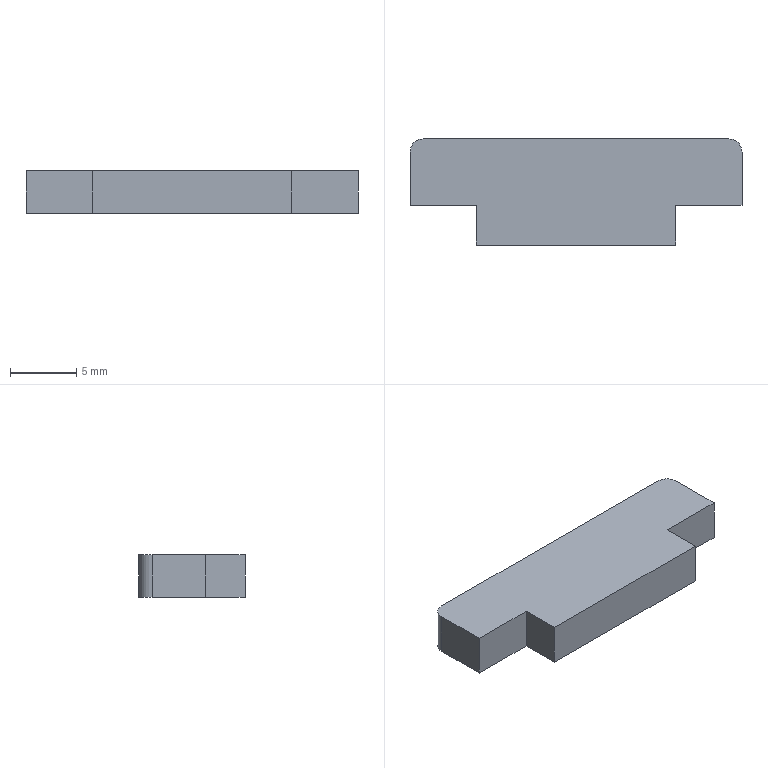Part | SolidWorks | features FlatPattern 1, SMBaseFlange 1, SheetMetal 1 | 1 solid | 12 faces | box 25 x 8 x 3.2 mm | volume 542.627 mm3 | plane 10 | cylinder 2 | commonest cylinder face diameters 2 x2
STEP:
#1=CARTESIAN_POINT('',(100.,-30.,0.));
#2=VERTEX_POINT('',#1);
#3=CARTESIAN_POINT('',(100.,-34.,0.));
#4=VERTEX_POINT('',#3);
#5=CARTESIAN_POINT('',(100.,-34.,0.));
#6=DIRECTION('',(0.,-1.,0.));
#7=VECTOR('',#6,1000.);
#8=LINE('',#5,#7);
#9=EDGE_CURVE('',#2,#4,#8,.T.);
#10=ORIENTED_EDGE('',*,*,#9,.T.);
#11=CARTESIAN_POINT('',(100.,-34.,3.2));
#12=VERTEX_POINT('',#11);
#13=CARTESIAN_POINT('',(100.,-34.,3.2));
#14=DIRECTION('',(0.,0.,-1.));
#15=VECTOR('',#14,1000.);
#16=LINE('',#13,#15);
#17=EDGE_CURVE('',#12,#4,#16,.T.);
#18=ORIENTED_EDGE('',*,*,#17,.F.);
#19=CARTESIAN_POINT('',(100.,-30.,3.2));
#20=VERTEX_POINT('',#19);
#21=CARTESIAN_POINT('',(100.,-34.,3.2));
#22=DIRECTION('',(0.,-1.,0.));
#23=VECTOR('',#22,1000.);
#24=LINE('',#21,#23);
#25=EDGE_CURVE('',#20,#12,#24,.T.);
#26=ORIENTED_EDGE('',*,*,#25,.F.);
#27=CARTESIAN_POINT('',(100.,-30.,3.2));
#28=DIRECTION('',(0.,0.,-1.));
#29=VECTOR('',#28,1000.);
#30=LINE('',#27,#29);
#31=EDGE_CURVE('',#20,#2,#30,.T.);
#32=ORIENTED_EDGE('',*,*,#31,.T.);
#33=EDGE_LOOP('',(#10,#18,#26,#32));
#34=FACE_OUTER_BOUND('',#33,.T.);
#35=CARTESIAN_POINT('',(100.,-34.,3.2));
#36=DIRECTION('',(1.,0.,0.));
#37=DIRECTION('',(0.,0.,-1.));
#38=AXIS2_PLACEMENT_3D('',#35,#36,#37);
#39=PLANE('',#38);
#40=ADVANCED_FACE('',(#34),#39,.F.);
#41=CARTESIAN_POINT('',(105.,-34.,0.));
#42=VERTEX_POINT('',#41);
#43=CARTESIAN_POINT('',(100.,-34.,0.));
#44=DIRECTION('',(1.,0.,0.));
#45=VECTOR('',#44,1000.);
#46=LINE('',#43,#45);
#47=EDGE_CURVE('',#4,#42,#46,.T.);
#48=ORIENTED_EDGE('',*,*,#47,.T.);
#49=CARTESIAN_POINT('',(105.,-34.,3.2));
#50=VERTEX_POINT('',#49);
#51=CARTESIAN_POINT('',(105.,-34.,3.2));
#52=DIRECTION('',(0.,0.,-1.));
#53=VECTOR('',#52,1000.);
#54=LINE('',#51,#53);
#55=EDGE_CURVE('',#50,#42,#54,.T.);
#56=ORIENTED_EDGE('',*,*,#55,.F.);
#57=CARTESIAN_POINT('',(100.,-34.,3.2));
#58=DIRECTION('',(1.,0.,0.));
#59=VECTOR('',#58,1000.);
#60=LINE('',#57,#59);
#61=EDGE_CURVE('',#12,#50,#60,.T.);
#62=ORIENTED_EDGE('',*,*,#61,.F.);
#63=ORIENTED_EDGE('',*,*,#17,.T.);
#64=EDGE_LOOP('',(#48,#56,#62,#63));
#65=FACE_OUTER_BOUND('',#64,.T.);
#66=CARTESIAN_POINT('',(100.,-34.,3.2));
#67=DIRECTION('',(0.,1.,0.));
#68=DIRECTION('',(0.,0.,1.));
#69=AXIS2_PLACEMENT_3D('',#66,#67,#68);
#70=PLANE('',#69);
#71=ADVANCED_FACE('',(#65),#70,.F.);
#72=CARTESIAN_POINT('',(105.,-37.,0.));
#73=VERTEX_POINT('',#72);
#74=CARTESIAN_POINT('',(105.,-34.,0.));
#75=DIRECTION('',(0.,-1.,0.));
#76=VECTOR('',#75,1000.);
#77=LINE('',#74,#76);
#78=EDGE_CURVE('',#42,#73,#77,.T.);
#79=ORIENTED_EDGE('',*,*,#78,.T.);
#80=CARTESIAN_POINT('',(105.,-37.,3.2));
#81=VERTEX_POINT('',#80);
#82=CARTESIAN_POINT('',(105.,-37.,3.2));
#83=DIRECTION('',(0.,0.,-1.));
#84=VECTOR('',#83,1000.);
#85=LINE('',#82,#84);
#86=EDGE_CURVE('',#81,#73,#85,.T.);
#87=ORIENTED_EDGE('',*,*,#86,.F.);
#88=CARTESIAN_POINT('',(105.,-34.,3.2));
#89=DIRECTION('',(0.,-1.,0.));
#90=VECTOR('',#89,1000.);
#91=LINE('',#88,#90);
#92=EDGE_CURVE('',#50,#81,#91,.T.);
#93=ORIENTED_EDGE('',*,*,#92,.F.);
#94=ORIENTED_EDGE('',*,*,#55,.T.);
#95=EDGE_LOOP('',(#79,#87,#93,#94));
#96=FACE_OUTER_BOUND('',#95,.T.);
#97=CARTESIAN_POINT('',(105.,-34.,3.2));
#98=DIRECTION('',(1.,0.,0.));
#99=DIRECTION('',(0.,0.,-1.));
#100=AXIS2_PLACEMENT_3D('',#97,#98,#99);
#101=PLANE('',#100);
#102=ADVANCED_FACE('',(#96),#101,.F.);
#103=CARTESIAN_POINT('',(120.,-37.,0.));
#104=VERTEX_POINT('',#103);
#105=CARTESIAN_POINT('',(105.,-37.,0.));
#106=DIRECTION('',(1.,0.,0.));
#107=VECTOR('',#106,1000.);
#108=LINE('',#105,#107);
#109=EDGE_CURVE('',#73,#104,#108,.T.);
#110=ORIENTED_EDGE('',*,*,#109,.T.);
#111=CARTESIAN_POINT('',(120.,-37.,3.2));
#112=VERTEX_POINT('',#111);
#113=CARTESIAN_POINT('',(120.,-37.,3.2));
#114=DIRECTION('',(0.,0.,-1.));
#115=VECTOR('',#114,1000.);
#116=LINE('',#113,#115);
#117=EDGE_CURVE('',#112,#104,#116,.T.);
#118=ORIENTED_EDGE('',*,*,#117,.F.);
#119=CARTESIAN_POINT('',(105.,-37.,3.2));
#120=DIRECTION('',(1.,0.,0.));
#121=VECTOR('',#120,1000.);
#122=LINE('',#119,#121);
#123=EDGE_CURVE('',#81,#112,#122,.T.);
#124=ORIENTED_EDGE('',*,*,#123,.F.);
#125=ORIENTED_EDGE('',*,*,#86,.T.);
#126=EDGE_LOOP('',(#110,#118,#124,#125));
#127=FACE_OUTER_BOUND('',#126,.T.);
#128=CARTESIAN_POINT('',(105.,-37.,3.2));
#129=DIRECTION('',(0.,1.,0.));
#130=DIRECTION('',(0.,0.,1.));
#131=AXIS2_PLACEMENT_3D('',#128,#129,#130);
#132=PLANE('',#131);
#133=ADVANCED_FACE('',(#127),#132,.F.);
#134=CARTESIAN_POINT('',(120.,-34.,0.));
#135=VERTEX_POINT('',#134);
#136=CARTESIAN_POINT('',(120.,-37.,0.));
#137=DIRECTION('',(0.,1.,0.));
#138=VECTOR('',#137,1000.);
#139=LINE('',#136,#138);
#140=EDGE_CURVE('',#104,#135,#139,.T.);
#141=ORIENTED_EDGE('',*,*,#140,.T.);
#142=CARTESIAN_POINT('',(120.,-34.,3.2));
#143=VERTEX_POINT('',#142);
#144=CARTESIAN_POINT('',(120.,-34.,3.2));
#145=DIRECTION('',(0.,0.,-1.));
#146=VECTOR('',#145,1000.);
#147=LINE('',#144,#146);
#148=EDGE_CURVE('',#143,#135,#147,.T.);
#149=ORIENTED_EDGE('',*,*,#148,.F.);
#150=CARTESIAN_POINT('',(120.,-37.,3.2));
#151=DIRECTION('',(0.,1.,0.));
#152=VECTOR('',#151,1000.);
#153=LINE('',#150,#152);
#154=EDGE_CURVE('',#112,#143,#153,.T.);
#155=ORIENTED_EDGE('',*,*,#154,.F.);
#156=ORIENTED_EDGE('',*,*,#117,.T.);
#157=EDGE_LOOP('',(#141,#149,#155,#156));
#158=FACE_OUTER_BOUND('',#157,.T.);
#159=CARTESIAN_POINT('',(120.,-37.,3.2));
#160=DIRECTION('',(-1.,0.,0.));
#161=DIRECTION('',(0.,0.,1.));
#162=AXIS2_PLACEMENT_3D('',#159,#160,#161);
#163=PLANE('',#162);
#164=ADVANCED_FACE('',(#158),#163,.F.);
#165=CARTESIAN_POINT('',(125.,-34.,0.));
#166=VERTEX_POINT('',#165);
#167=CARTESIAN_POINT('',(120.,-34.,0.));
#168=DIRECTION('',(1.,0.,0.));
#169=VECTOR('',#168,1000.);
#170=LINE('',#167,#169);
#171=EDGE_CURVE('',#135,#166,#170,.T.);
#172=ORIENTED_EDGE('',*,*,#171,.T.);
#173=CARTESIAN_POINT('',(125.,-34.,3.2));
#174=VERTEX_POINT('',#173);
#175=CARTESIAN_POINT('',(125.,-34.,3.2));
#176=DIRECTION('',(0.,0.,-1.));
#177=VECTOR('',#176,1000.);
#178=LINE('',#175,#177);
#179=EDGE_CURVE('',#174,#166,#178,.T.);
#180=ORIENTED_EDGE('',*,*,#179,.F.);
#181=CARTESIAN_POINT('',(120.,-34.,3.2));
#182=DIRECTION('',(1.,0.,0.));
#183=VECTOR('',#182,1000.);
#184=LINE('',#181,#183);
#185=EDGE_CURVE('',#143,#174,#184,.T.);
#186=ORIENTED_EDGE('',*,*,#185,.F.);
#187=ORIENTED_EDGE('',*,*,#148,.T.);
#188=EDGE_LOOP('',(#172,#180,#186,#187));
#189=FACE_OUTER_BOUND('',#188,.T.);
#190=CARTESIAN_POINT('',(120.,-34.,3.2));
#191=DIRECTION('',(0.,1.,0.));
#192=DIRECTION('',(0.,0.,1.));
#193=AXIS2_PLACEMENT_3D('',#190,#191,#192);
#194=PLANE('',#193);
#195=ADVANCED_FACE('',(#189),#194,.F.);
#196=CARTESIAN_POINT('',(125.,-30.,0.));
#197=VERTEX_POINT('',#196);
#198=CARTESIAN_POINT('',(125.,-34.,0.));
#199=DIRECTION('',(0.,1.,0.));
#200=VECTOR('',#199,1000.);
#201=LINE('',#198,#200);
#202=EDGE_CURVE('',#166,#197,#201,.T.);
#203=ORIENTED_EDGE('',*,*,#202,.T.);
#204=CARTESIAN_POINT('',(125.,-30.,3.2));
#205=VERTEX_POINT('',#204);
#206=CARTESIAN_POINT('',(125.,-30.,3.2));
#207=DIRECTION('',(0.,0.,-1.));
#208=VECTOR('',#207,1000.);
#209=LINE('',#206,#208);
#210=EDGE_CURVE('',#205,#197,#209,.T.);
#211=ORIENTED_EDGE('',*,*,#210,.F.);
#212=CARTESIAN_POINT('',(125.,-34.,3.2));
#213=DIRECTION('',(0.,1.,0.));
#214=VECTOR('',#213,1000.);
#215=LINE('',#212,#214);
#216=EDGE_CURVE('',#174,#205,#215,.T.);
#217=ORIENTED_EDGE('',*,*,#216,.F.);
#218=ORIENTED_EDGE('',*,*,#179,.T.);
#219=EDGE_LOOP('',(#203,#211,#217,#218));
#220=FACE_OUTER_BOUND('',#219,.T.);
#221=CARTESIAN_POINT('',(125.,-34.,3.2));
#222=DIRECTION('',(-1.,0.,0.));
#223=DIRECTION('',(0.,0.,1.));
#224=AXIS2_PLACEMENT_3D('',#221,#222,#223);
#225=PLANE('',#224);
#226=ADVANCED_FACE('',(#220),#225,.F.);
#227=CARTESIAN_POINT('',(124.,-29.,0.));
#228=VERTEX_POINT('',#227);
#229=CARTESIAN_POINT('',(124.,-30.,0.));
#230=DIRECTION('',(0.,0.,1.));
#231=DIRECTION('',(-1.,0.,0.));
#232=AXIS2_PLACEMENT_3D('',#229,#230,#231);
#233=CIRCLE('',#232,1.);
#234=EDGE_CURVE('',#197,#228,#233,.T.);
#235=ORIENTED_EDGE('',*,*,#234,.T.);
#236=CARTESIAN_POINT('',(124.,-29.,3.2));
#237=VERTEX_POINT('',#236);
#238=CARTESIAN_POINT('',(124.,-29.,3.2));
#239=DIRECTION('',(0.,0.,-1.));
#240=VECTOR('',#239,1000.);
#241=LINE('',#238,#240);
#242=EDGE_CURVE('',#237,#228,#241,.T.);
#243=ORIENTED_EDGE('',*,*,#242,.F.);
#244=CARTESIAN_POINT('',(124.,-30.,3.2));
#245=DIRECTION('',(0.,0.,1.));
#246=DIRECTION('',(-1.,0.,0.));
#247=AXIS2_PLACEMENT_3D('',#244,#245,#246);
#248=CIRCLE('',#247,1.);
#249=EDGE_CURVE('',#205,#237,#248,.T.);
#250=ORIENTED_EDGE('',*,*,#249,.F.);
#251=ORIENTED_EDGE('',*,*,#210,.T.);
#252=EDGE_LOOP('',(#235,#243,#250,#251));
#253=FACE_OUTER_BOUND('',#252,.T.);
#254=CARTESIAN_POINT('',(124.,-30.,3.2));
#255=DIRECTION('',(0.,0.,-1.));
#256=DIRECTION('',(-1.,0.,0.));
#257=AXIS2_PLACEMENT_3D('',#254,#255,#256);
#258=CYLINDRICAL_SURFACE('',#257,1.);
#259=ADVANCED_FACE('',(#253),#258,.T.);
#260=CARTESIAN_POINT('',(101.,-29.,0.));
#261=VERTEX_POINT('',#260);
#262=CARTESIAN_POINT('',(101.,-29.,0.));
#263=DIRECTION('',(-1.,0.,0.));
#264=VECTOR('',#263,1000.);
#265=LINE('',#262,#264);
#266=EDGE_CURVE('',#228,#261,#265,.T.);
#267=ORIENTED_EDGE('',*,*,#266,.T.);
#268=CARTESIAN_POINT('',(101.,-29.,3.2));
#269=VERTEX_POINT('',#268);
#270=CARTESIAN_POINT('',(101.,-29.,3.2));
#271=DIRECTION('',(0.,0.,-1.));
#272=VECTOR('',#271,1000.);
#273=LINE('',#270,#272);
#274=EDGE_CURVE('',#269,#261,#273,.T.);
#275=ORIENTED_EDGE('',*,*,#274,.F.);
#276=CARTESIAN_POINT('',(101.,-29.,3.2));
#277=DIRECTION('',(-1.,0.,0.));
#278=VECTOR('',#277,1000.);
#279=LINE('',#276,#278);
#280=EDGE_CURVE('',#237,#269,#279,.T.);
#281=ORIENTED_EDGE('',*,*,#280,.F.);
#282=ORIENTED_EDGE('',*,*,#242,.T.);
#283=EDGE_LOOP('',(#267,#275,#281,#282));
#284=FACE_OUTER_BOUND('',#283,.T.);
#285=CARTESIAN_POINT('',(101.,-29.,3.2));
#286=DIRECTION('',(0.,-1.,0.));
#287=DIRECTION('',(0.,0.,-1.));
#288=AXIS2_PLACEMENT_3D('',#285,#286,#287);
#289=PLANE('',#288);
#290=ADVANCED_FACE('',(#284),#289,.F.);
#291=CARTESIAN_POINT('',(101.,-30.,0.));
#292=DIRECTION('',(0.,0.,1.));
#293=DIRECTION('',(-1.,0.,0.));
#294=AXIS2_PLACEMENT_3D('',#291,#292,#293);
#295=CIRCLE('',#294,1.);
#296=EDGE_CURVE('',#261,#2,#295,.T.);
#297=ORIENTED_EDGE('',*,*,#296,.T.);
#298=ORIENTED_EDGE('',*,*,#31,.F.);
#299=CARTESIAN_POINT('',(101.,-30.,3.2));
#300=DIRECTION('',(0.,0.,1.));
#301=DIRECTION('',(-1.,0.,0.));
#302=AXIS2_PLACEMENT_3D('',#299,#300,#301);
#303=CIRCLE('',#302,1.);
#304=EDGE_CURVE('',#269,#20,#303,.T.);
#305=ORIENTED_EDGE('',*,*,#304,.F.);
#306=ORIENTED_EDGE('',*,*,#274,.T.);
#307=EDGE_LOOP('',(#297,#298,#305,#306));
#308=FACE_OUTER_BOUND('',#307,.T.);
#309=CARTESIAN_POINT('',(101.,-30.,3.2));
#310=DIRECTION('',(0.,0.,-1.));
#311=DIRECTION('',(-1.,0.,0.));
#312=AXIS2_PLACEMENT_3D('',#309,#310,#311);
#313=CYLINDRICAL_SURFACE('',#312,1.);
#314=ADVANCED_FACE('',(#308),#313,.T.);
#315=ORIENTED_EDGE('',*,*,#25,.T.);
#316=ORIENTED_EDGE('',*,*,#61,.T.);
#317=ORIENTED_EDGE('',*,*,#92,.T.);
#318=ORIENTED_EDGE('',*,*,#123,.T.);
#319=ORIENTED_EDGE('',*,*,#154,.T.);
#320=ORIENTED_EDGE('',*,*,#185,.T.);
#321=ORIENTED_EDGE('',*,*,#216,.T.);
#322=ORIENTED_EDGE('',*,*,#249,.T.);
#323=ORIENTED_EDGE('',*,*,#280,.T.);
#324=ORIENTED_EDGE('',*,*,#304,.T.);
#325=EDGE_LOOP('',(#315,#316,#317,#318,#319,#320,#321,#322,#323,#324));
#326=FACE_OUTER_BOUND('',#325,.T.);
#327=CARTESIAN_POINT('',(101.,-30.,3.2));
#328=DIRECTION('',(0.,0.,-1.));
#329=DIRECTION('',(-1.,0.,0.));
#330=AXIS2_PLACEMENT_3D('',#327,#328,#329);
#331=PLANE('',#330);
#332=ADVANCED_FACE('',(#326),#331,.F.);
#333=ORIENTED_EDGE('',*,*,#9,.F.);
#334=ORIENTED_EDGE('',*,*,#296,.F.);
#335=ORIENTED_EDGE('',*,*,#266,.F.);
#336=ORIENTED_EDGE('',*,*,#234,.F.);
#337=ORIENTED_EDGE('',*,*,#202,.F.);
#338=ORIENTED_EDGE('',*,*,#171,.F.);
#339=ORIENTED_EDGE('',*,*,#140,.F.);
#340=ORIENTED_EDGE('',*,*,#109,.F.);
#341=ORIENTED_EDGE('',*,*,#78,.F.);
#342=ORIENTED_EDGE('',*,*,#47,.F.);
#343=EDGE_LOOP('',(#333,#334,#335,#336,#337,#338,#339,#340,#341,#342));
#344=FACE_OUTER_BOUND('',#343,.T.);
#345=CARTESIAN_POINT('',(101.,-30.,0.));
#346=DIRECTION('',(0.,0.,-1.));
#347=DIRECTION('',(-1.,0.,0.));
#348=AXIS2_PLACEMENT_3D('',#345,#346,#347);
#349=PLANE('',#348);
#350=ADVANCED_FACE('',(#344),#349,.T.);
#351=CLOSED_SHELL('',(#40,#71,#102,#133,#164,#195,#226,#259,#290,#314,#332,#350));
#352=MANIFOLD_SOLID_BREP('',#351);
#353=CARTESIAN_POINT('',(0.,0.,0.));
#354=DIRECTION('',(0.,0.,1.));
#355=DIRECTION('',(1.,0.,0.));
#356=AXIS2_PLACEMENT_3D('',#353,#354,#355);
#357=(LENGTH_UNIT()NAMED_UNIT(*)SI_UNIT(.MILLI.,.METRE.));
#358=UNCERTAINTY_MEASURE_WITH_UNIT(LENGTH_MEASURE(0.00001),#357,'','');
#359=(NAMED_UNIT(*)PLANE_ANGLE_UNIT()SI_UNIT($,.RADIAN.));
#360=(NAMED_UNIT(*)SI_UNIT($,.STERADIAN.)SOLID_ANGLE_UNIT());
#361=(GEOMETRIC_REPRESENTATION_CONTEXT(3)GLOBAL_UNCERTAINTY_ASSIGNED_CONTEXT((#358))GLOBAL_UNIT_ASSIGNED_CONTEXT((#357,#359,#360))REPRESENTATION_CONTEXT('',''));
#362=ADVANCED_BREP_SHAPE_REPRESENTATION('',(#352,#356),#361);